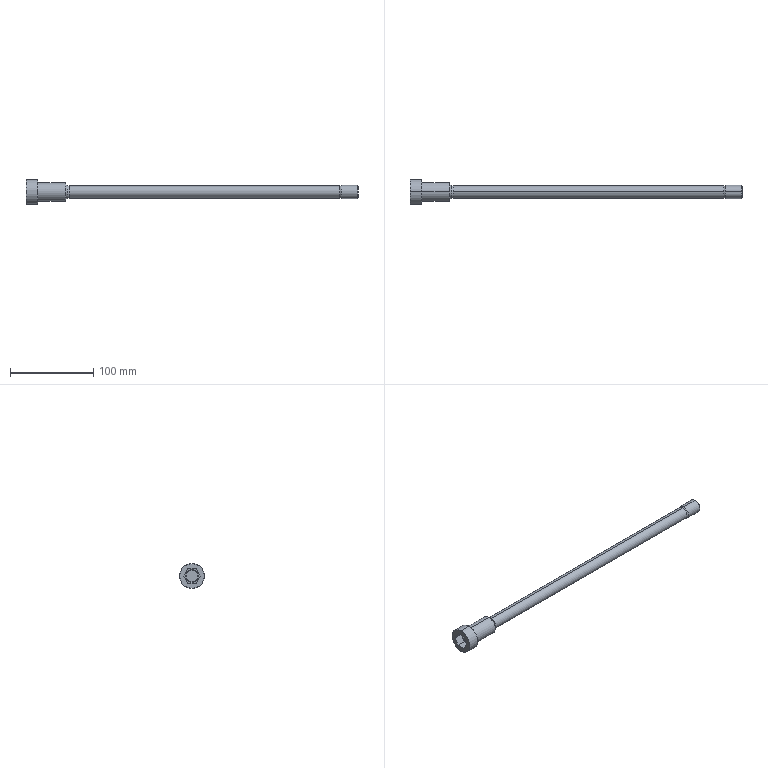Part | STEP file | SI160_250 | 1 solid | 38 faces | box 400 x 30 x 30 mm | volume 76937 mm3 | cone 14 | cylinder 12 | plane 12 | commonest cylinder face diameters 16 x4 13.835 x2 14.6 x2 22 x2 30 x2